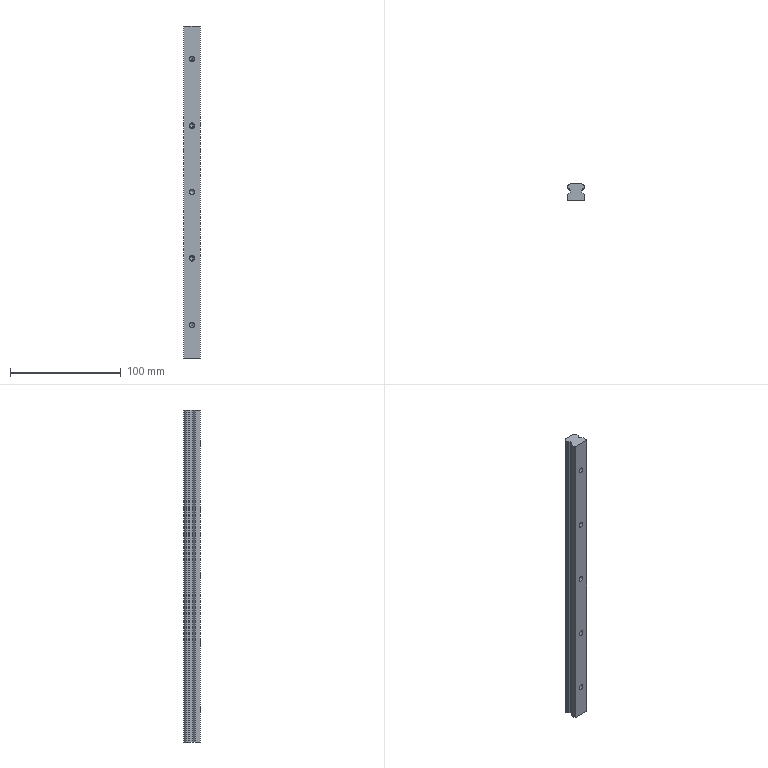Part | STEP file | 1 solid | 61 faces | box 15 x 15 x 300 mm | volume 59817 mm3 | cylinder 26 | plane 25 | cone 10 | commonest cylinder face diameters 4.25 x10 5 x10 1.459 x6